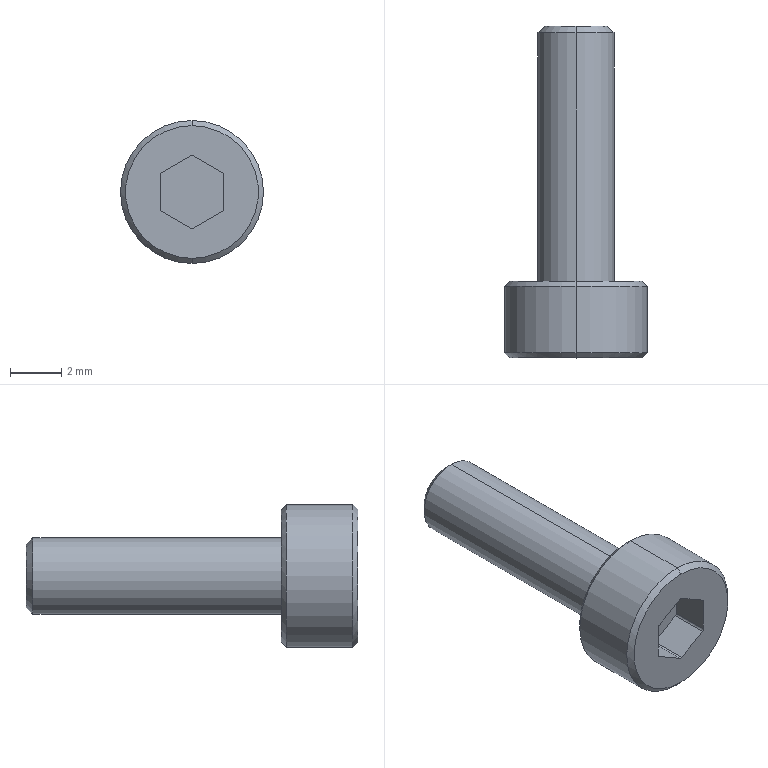Part | SolidWorks | features Chamfer 1, Extrusion 1, Fillet 1, ICE 1, StudWizard 1 | 1 solid | 27 faces | box 5.6 x 13 x 5.6 mm | volume 135.451 mm3 | cylinder 11 | plane 10 | cone 6 | commonest cylinder face diameters 0.2 x7 3 x2 5.6 x2
STEP:
#1=CARTESIAN_POINT('',(0.,0.,1.428));
#2=VERTEX_POINT('',#1);
#3=CARTESIAN_POINT('',(0.05,0.,1.415));
#4=VERTEX_POINT('',#3);
#5=CARTESIAN_POINT('',(0.,0.,1.328));
#6=DIRECTION('',(0.,1.,0.));
#7=DIRECTION('',(0.,0.,1.));
#8=AXIS2_PLACEMENT_3D('',#5,#6,#7);
#9=CIRCLE('',#8,0.1);
#10=EDGE_CURVE('',#2,#4,#9,.T.);
#11=ORIENTED_EDGE('',*,*,#10,.F.);
#12=CARTESIAN_POINT('',(0.,1.5,1.428));
#13=VERTEX_POINT('',#12);
#14=CARTESIAN_POINT('',(0.,1.5,1.428));
#15=DIRECTION('',(0.,1.,0.));
#16=VECTOR('',#15,1000.);
#17=LINE('',#14,#16);
#18=EDGE_CURVE('',#2,#13,#17,.T.);
#19=ORIENTED_EDGE('',*,*,#18,.T.);
#20=CARTESIAN_POINT('',(0.05,1.5,1.415));
#21=VERTEX_POINT('',#20);
#22=CARTESIAN_POINT('',(0.,1.5,1.328));
#23=DIRECTION('',(0.,-1.,0.));
#24=DIRECTION('',(0.,0.,-1.));
#25=AXIS2_PLACEMENT_3D('',#22,#23,#24);
#26=CIRCLE('',#25,0.1);
#27=EDGE_CURVE('',#21,#13,#26,.T.);
#28=ORIENTED_EDGE('',*,*,#27,.F.);
#29=CARTESIAN_POINT('',(0.05,1.5,1.415));
#30=DIRECTION('',(0.,1.,0.));
#31=VECTOR('',#30,1000.);
#32=LINE('',#29,#31);
#33=EDGE_CURVE('',#4,#21,#32,.T.);
#34=ORIENTED_EDGE('',*,*,#33,.F.);
#35=EDGE_LOOP('',(#11,#19,#28,#34));
#36=FACE_OUTER_BOUND('',#35,.T.);
#37=CARTESIAN_POINT('',(0.,1.5,1.328));
#38=DIRECTION('',(0.,1.,0.));
#39=DIRECTION('',(0.,0.,1.));
#40=AXIS2_PLACEMENT_3D('',#37,#38,#39);
#41=CYLINDRICAL_SURFACE('',#40,0.1);
#42=ADVANCED_FACE('',(#36),#41,.F.);
#43=CARTESIAN_POINT('',(0.,0.,-2.6));
#44=VERTEX_POINT('',#43);
#45=CARTESIAN_POINT('',(0.,0.,2.6));
#46=VERTEX_POINT('',#45);
#47=CARTESIAN_POINT('',(0.,0.,0.));
#48=DIRECTION('',(0.,-1.,0.));
#49=DIRECTION('',(0.,0.,1.));
#50=AXIS2_PLACEMENT_3D('',#47,#48,#49);
#51=CIRCLE('',#50,2.6);
#52=EDGE_CURVE('',#44,#46,#51,.T.);
#53=ORIENTED_EDGE('',*,*,#52,.F.);
#54=CARTESIAN_POINT('',(0.,0.2,-2.8));
#55=VERTEX_POINT('',#54);
#56=CARTESIAN_POINT('',(0.,0.2,-2.8));
#57=DIRECTION('',(0.,0.7071,-0.7071));
#58=VECTOR('',#57,1000.);
#59=LINE('',#56,#58);
#60=EDGE_CURVE('',#44,#55,#59,.T.);
#61=ORIENTED_EDGE('',*,*,#60,.T.);
#62=CARTESIAN_POINT('',(0.,0.2,2.8));
#63=VERTEX_POINT('',#62);
#64=CARTESIAN_POINT('',(0.,0.2,0.));
#65=DIRECTION('',(0.,1.,0.));
#66=DIRECTION('',(0.,0.,1.));
#67=AXIS2_PLACEMENT_3D('',#64,#65,#66);
#68=CIRCLE('',#67,2.8);
#69=EDGE_CURVE('',#63,#55,#68,.T.);
#70=ORIENTED_EDGE('',*,*,#69,.F.);
#71=CARTESIAN_POINT('',(0.,0.2,2.8));
#72=DIRECTION('',(0.,0.7071,0.7071));
#73=VECTOR('',#72,1000.);
#74=LINE('',#71,#73);
#75=EDGE_CURVE('',#46,#63,#74,.T.);
#76=ORIENTED_EDGE('',*,*,#75,.F.);
#77=EDGE_LOOP('',(#53,#61,#70,#76));
#78=FACE_OUTER_BOUND('',#77,.T.);
#79=CARTESIAN_POINT('',(0.,0.2,0.));
#80=DIRECTION('',(0.,1.,0.));
#81=DIRECTION('',(0.,0.,1.));
#82=AXIS2_PLACEMENT_3D('',#79,#80,#81);
#83=CONICAL_SURFACE('',#82,2.8,0.7854);
#84=ADVANCED_FACE('',(#78),#83,.T.);
#85=CARTESIAN_POINT('',(0.,3.,2.6));
#86=VERTEX_POINT('',#85);
#87=CARTESIAN_POINT('',(0.,3.,-2.6));
#88=VERTEX_POINT('',#87);
#89=CARTESIAN_POINT('',(0.,3.,0.));
#90=DIRECTION('',(0.,1.,0.));
#91=DIRECTION('',(0.,0.,1.));
#92=AXIS2_PLACEMENT_3D('',#89,#90,#91);
#93=CIRCLE('',#92,2.6);
#94=EDGE_CURVE('',#86,#88,#93,.T.);
#95=ORIENTED_EDGE('',*,*,#94,.F.);
#96=CARTESIAN_POINT('',(0.,2.8,2.8));
#97=VERTEX_POINT('',#96);
#98=CARTESIAN_POINT('',(0.,3.,2.6));
#99=DIRECTION('',(0.,-0.7071,0.7071));
#100=VECTOR('',#99,1000.);
#101=LINE('',#98,#100);
#102=EDGE_CURVE('',#86,#97,#101,.T.);
#103=ORIENTED_EDGE('',*,*,#102,.T.);
#104=CARTESIAN_POINT('',(0.,2.8,-2.8));
#105=VERTEX_POINT('',#104);
#106=CARTESIAN_POINT('',(0.,2.8,0.));
#107=DIRECTION('',(0.,-1.,0.));
#108=DIRECTION('',(0.,0.,1.));
#109=AXIS2_PLACEMENT_3D('',#106,#107,#108);
#110=CIRCLE('',#109,2.8);
#111=EDGE_CURVE('',#105,#97,#110,.T.);
#112=ORIENTED_EDGE('',*,*,#111,.F.);
#113=CARTESIAN_POINT('',(0.,3.,-2.6));
#114=DIRECTION('',(0.,-0.7071,-0.7071));
#115=VECTOR('',#114,1000.);
#116=LINE('',#113,#115);
#117=EDGE_CURVE('',#88,#105,#116,.T.);
#118=ORIENTED_EDGE('',*,*,#117,.F.);
#119=EDGE_LOOP('',(#95,#103,#112,#118));
#120=FACE_OUTER_BOUND('',#119,.T.);
#121=CARTESIAN_POINT('',(0.,3.,0.));
#122=DIRECTION('',(0.,-1.,0.));
#123=DIRECTION('',(0.,0.,-1.));
#124=AXIS2_PLACEMENT_3D('',#121,#122,#123);
#125=CONICAL_SURFACE('',#124,2.6,0.7854);
#126=ADVANCED_FACE('',(#120),#125,.T.);
#127=CARTESIAN_POINT('',(0.,12.73,-1.5));
#128=VERTEX_POINT('',#127);
#129=CARTESIAN_POINT('',(0.,12.73,1.5));
#130=VERTEX_POINT('',#129);
#131=CARTESIAN_POINT('',(0.,12.73,0.));
#132=DIRECTION('',(0.,-1.,0.));
#133=DIRECTION('',(0.,0.,-1.));
#134=AXIS2_PLACEMENT_3D('',#131,#132,#133);
#135=CIRCLE('',#134,1.5);
#136=EDGE_CURVE('',#128,#130,#135,.T.);
#137=ORIENTED_EDGE('',*,*,#136,.T.);
#138=CARTESIAN_POINT('',(0.,3.,1.5));
#139=VERTEX_POINT('',#138);
#140=CARTESIAN_POINT('',(0.,3.,1.5));
#141=DIRECTION('',(0.,-1.,0.));
#142=VECTOR('',#141,1000.);
#143=LINE('',#140,#142);
#144=EDGE_CURVE('',#130,#139,#143,.T.);
#145=ORIENTED_EDGE('',*,*,#144,.T.);
#146=CARTESIAN_POINT('',(0.,3.,-1.5));
#147=VERTEX_POINT('',#146);
#148=CARTESIAN_POINT('',(0.,3.,0.));
#149=DIRECTION('',(0.,-1.,0.));
#150=DIRECTION('',(0.,0.,-1.));
#151=AXIS2_PLACEMENT_3D('',#148,#149,#150);
#152=CIRCLE('',#151,1.5);
#153=EDGE_CURVE('',#147,#139,#152,.T.);
#154=ORIENTED_EDGE('',*,*,#153,.F.);
#155=CARTESIAN_POINT('',(0.,3.,-1.5));
#156=DIRECTION('',(0.,-1.,0.));
#157=VECTOR('',#156,1000.);
#158=LINE('',#155,#157);
#159=EDGE_CURVE('',#128,#147,#158,.T.);
#160=ORIENTED_EDGE('',*,*,#159,.F.);
#161=EDGE_LOOP('',(#137,#145,#154,#160));
#162=FACE_OUTER_BOUND('',#161,.T.);
#163=CARTESIAN_POINT('',(0.,3.,0.));
#164=DIRECTION('',(0.,-1.,0.));
#165=DIRECTION('',(0.,0.,-1.));
#166=AXIS2_PLACEMENT_3D('',#163,#164,#165);
#167=CYLINDRICAL_SURFACE('',#166,1.5);
#168=ADVANCED_FACE('',(#162),#167,.T.);
#169=CARTESIAN_POINT('',(0.,13.,-1.23));
#170=VERTEX_POINT('',#169);
#171=CARTESIAN_POINT('',(0.,13.,1.23));
#172=VERTEX_POINT('',#171);
#173=CARTESIAN_POINT('',(0.,13.,0.));
#174=DIRECTION('',(0.,-1.,0.));
#175=DIRECTION('',(0.,0.,-1.));
#176=AXIS2_PLACEMENT_3D('',#173,#174,#175);
#177=CIRCLE('',#176,1.23);
#178=EDGE_CURVE('',#170,#172,#177,.T.);
#179=ORIENTED_EDGE('',*,*,#178,.T.);
#180=CARTESIAN_POINT('',(0.,12.73,1.5));
#181=DIRECTION('',(0.,-0.7071,0.7071));
#182=VECTOR('',#181,1000.);
#183=LINE('',#180,#182);
#184=EDGE_CURVE('',#172,#130,#183,.T.);
#185=ORIENTED_EDGE('',*,*,#184,.T.);
#186=ORIENTED_EDGE('',*,*,#136,.F.);
#187=CARTESIAN_POINT('',(0.,12.73,-1.5));
#188=DIRECTION('',(0.,-0.7071,-0.7071));
#189=VECTOR('',#188,1000.);
#190=LINE('',#187,#189);
#191=EDGE_CURVE('',#170,#128,#190,.T.);
#192=ORIENTED_EDGE('',*,*,#191,.F.);
#193=EDGE_LOOP('',(#179,#185,#186,#192));
#194=FACE_OUTER_BOUND('',#193,.T.);
#195=CARTESIAN_POINT('',(0.,12.73,0.));
#196=DIRECTION('',(0.,-1.,0.));
#197=DIRECTION('',(0.,0.,-1.));
#198=AXIS2_PLACEMENT_3D('',#195,#196,#197);
#199=CONICAL_SURFACE('',#198,1.5,0.7854);
#200=ADVANCED_FACE('',(#194),#199,.T.);
#201=ORIENTED_EDGE('',*,*,#111,.T.);
#202=CARTESIAN_POINT('',(0.,3.,2.8));
#203=DIRECTION('',(0.,-1.,0.));
#204=VECTOR('',#203,1000.);
#205=LINE('',#202,#204);
#206=EDGE_CURVE('',#97,#63,#205,.T.);
#207=ORIENTED_EDGE('',*,*,#206,.T.);
#208=ORIENTED_EDGE('',*,*,#69,.T.);
#209=CARTESIAN_POINT('',(0.,3.,-2.8));
#210=DIRECTION('',(0.,-1.,0.));
#211=VECTOR('',#210,1000.);
#212=LINE('',#209,#211);
#213=EDGE_CURVE('',#105,#55,#212,.T.);
#214=ORIENTED_EDGE('',*,*,#213,.F.);
#215=EDGE_LOOP('',(#201,#207,#208,#214));
#216=FACE_OUTER_BOUND('',#215,.T.);
#217=CARTESIAN_POINT('',(0.,3.,0.));
#218=DIRECTION('',(0.,-1.,0.));
#219=DIRECTION('',(0.,0.,-1.));
#220=AXIS2_PLACEMENT_3D('',#217,#218,#219);
#221=CYLINDRICAL_SURFACE('',#220,2.8);
#222=ADVANCED_FACE('',(#216),#221,.T.);
#223=ORIENTED_EDGE('',*,*,#206,.F.);
#224=CARTESIAN_POINT('',(0.,2.8,0.));
#225=DIRECTION('',(0.,-1.,0.));
#226=DIRECTION('',(0.,0.,1.));
#227=AXIS2_PLACEMENT_3D('',#224,#225,#226);
#228=CIRCLE('',#227,2.8);
#229=EDGE_CURVE('',#97,#105,#228,.T.);
#230=ORIENTED_EDGE('',*,*,#229,.T.);
#231=ORIENTED_EDGE('',*,*,#213,.T.);
#232=CARTESIAN_POINT('',(0.,0.2,0.));
#233=DIRECTION('',(0.,1.,0.));
#234=DIRECTION('',(0.,0.,1.));
#235=AXIS2_PLACEMENT_3D('',#232,#233,#234);
#236=CIRCLE('',#235,2.8);
#237=EDGE_CURVE('',#55,#63,#236,.T.);
#238=ORIENTED_EDGE('',*,*,#237,.T.);
#239=EDGE_LOOP('',(#223,#230,#231,#238));
#240=FACE_OUTER_BOUND('',#239,.T.);
#241=CARTESIAN_POINT('',(0.,3.,0.));
#242=DIRECTION('',(0.,-1.,0.));
#243=DIRECTION('',(0.,0.,-1.));
#244=AXIS2_PLACEMENT_3D('',#241,#242,#243);
#245=CYLINDRICAL_SURFACE('',#244,2.8);
#246=ADVANCED_FACE('',(#240),#245,.T.);
#247=CARTESIAN_POINT('',(0.,3.,0.));
#248=DIRECTION('',(0.,1.,0.));
#249=DIRECTION('',(0.,0.,1.));
#250=AXIS2_PLACEMENT_3D('',#247,#248,#249);
#251=CIRCLE('',#250,2.6);
#252=EDGE_CURVE('',#88,#86,#251,.T.);
#253=ORIENTED_EDGE('',*,*,#252,.T.);
#254=ORIENTED_EDGE('',*,*,#94,.T.);
#255=EDGE_LOOP('',(#253,#254));
#256=FACE_OUTER_BOUND('',#255,.T.);
#257=ORIENTED_EDGE('',*,*,#153,.T.);
#258=CARTESIAN_POINT('',(0.,3.,0.));
#259=DIRECTION('',(0.,-1.,0.));
#260=DIRECTION('',(0.,0.,-1.));
#261=AXIS2_PLACEMENT_3D('',#258,#259,#260);
#262=CIRCLE('',#261,1.5);
#263=EDGE_CURVE('',#139,#147,#262,.T.);
#264=ORIENTED_EDGE('',*,*,#263,.T.);
#265=EDGE_LOOP('',(#257,#264));
#266=FACE_BOUND('',#265,.T.);
#267=CARTESIAN_POINT('',(0.,3.,0.));
#268=DIRECTION('',(0.,1.,0.));
#269=DIRECTION('',(0.,0.,1.));
#270=AXIS2_PLACEMENT_3D('',#267,#268,#269);
#271=PLANE('',#270);
#272=ADVANCED_FACE('',(#256,#266),#271,.T.);
#273=CARTESIAN_POINT('',(0.,0.,0.));
#274=DIRECTION('',(0.,-1.,0.));
#275=DIRECTION('',(0.,0.,1.));
#276=AXIS2_PLACEMENT_3D('',#273,#274,#275);
#277=CIRCLE('',#276,2.6);
#278=EDGE_CURVE('',#46,#44,#277,.T.);
#279=ORIENTED_EDGE('',*,*,#278,.T.);
#280=ORIENTED_EDGE('',*,*,#52,.T.);
#281=EDGE_LOOP('',(#279,#280));
#282=FACE_OUTER_BOUND('',#281,.T.);
#283=CARTESIAN_POINT('',(-0.05,0.,1.415));
#284=VERTEX_POINT('',#283);
#285=CARTESIAN_POINT('',(-1.2,0.,0.7506));
#286=VERTEX_POINT('',#285);
#287=CARTESIAN_POINT('',(0.,0.,1.443));
#288=DIRECTION('',(-0.866,0.,-0.5));
#289=VECTOR('',#288,1000.);
#290=LINE('',#287,#289);
#291=EDGE_CURVE('',#284,#286,#290,.T.);
#292=ORIENTED_EDGE('',*,*,#291,.F.);
#293=CARTESIAN_POINT('',(0.,0.,1.328));
#294=DIRECTION('',(0.,1.,0.));
#295=DIRECTION('',(0.,0.,1.));
#296=AXIS2_PLACEMENT_3D('',#293,#294,#295);
#297=CIRCLE('',#296,0.1);
#298=EDGE_CURVE('',#284,#2,#297,.T.);
#299=ORIENTED_EDGE('',*,*,#298,.T.);
#300=ORIENTED_EDGE('',*,*,#10,.T.);
#301=CARTESIAN_POINT('',(1.2,0.,0.7506));
#302=VERTEX_POINT('',#301);
#303=CARTESIAN_POINT('',(1.25,0.,0.7217));
#304=DIRECTION('',(-0.866,0.,0.5));
#305=VECTOR('',#304,1000.);
#306=LINE('',#303,#305);
#307=EDGE_CURVE('',#302,#4,#306,.T.);
#308=ORIENTED_EDGE('',*,*,#307,.F.);
#309=CARTESIAN_POINT('',(1.25,0.,0.664));
#310=VERTEX_POINT('',#309);
#311=CARTESIAN_POINT('',(1.15,0.,0.664));
#312=DIRECTION('',(0.,1.,0.));
#313=DIRECTION('',(0.,0.,1.));
#314=AXIS2_PLACEMENT_3D('',#311,#312,#313);
#315=CIRCLE('',#314,0.1);
#316=EDGE_CURVE('',#302,#310,#315,.T.);
#317=ORIENTED_EDGE('',*,*,#316,.T.);
#318=CARTESIAN_POINT('',(1.25,0.,-0.664));
#319=VERTEX_POINT('',#318);
#320=CARTESIAN_POINT('',(1.25,0.,-0.7217));
#321=DIRECTION('',(0.,0.,1.));
#322=VECTOR('',#321,1000.);
#323=LINE('',#320,#322);
#324=EDGE_CURVE('',#319,#310,#323,.T.);
#325=ORIENTED_EDGE('',*,*,#324,.F.);
#326=CARTESIAN_POINT('',(1.2,0.,-0.7506));
#327=VERTEX_POINT('',#326);
#328=CARTESIAN_POINT('',(1.15,0.,-0.664));
#329=DIRECTION('',(0.,1.,0.));
#330=DIRECTION('',(0.,0.,1.));
#331=AXIS2_PLACEMENT_3D('',#328,#329,#330);
#332=CIRCLE('',#331,0.1);
#333=EDGE_CURVE('',#319,#327,#332,.T.);
#334=ORIENTED_EDGE('',*,*,#333,.T.);
#335=CARTESIAN_POINT('',(0.05,0.,-1.415));
#336=VERTEX_POINT('',#335);
#337=CARTESIAN_POINT('',(0.,0.,-1.443));
#338=DIRECTION('',(0.866,0.,0.5));
#339=VECTOR('',#338,1000.);
#340=LINE('',#337,#339);
#341=EDGE_CURVE('',#336,#327,#340,.T.);
#342=ORIENTED_EDGE('',*,*,#341,.F.);
#343=CARTESIAN_POINT('',(-0.05,0.,-1.415));
#344=VERTEX_POINT('',#343);
#345=CARTESIAN_POINT('',(0.,0.,-1.328));
#346=DIRECTION('',(0.,1.,0.));
#347=DIRECTION('',(0.,0.,1.));
#348=AXIS2_PLACEMENT_3D('',#345,#346,#347);
#349=CIRCLE('',#348,0.1);
#350=EDGE_CURVE('',#336,#344,#349,.T.);
#351=ORIENTED_EDGE('',*,*,#350,.T.);
#352=CARTESIAN_POINT('',(-1.2,0.,-0.7506));
#353=VERTEX_POINT('',#352);
#354=CARTESIAN_POINT('',(-1.25,0.,-0.7217));
#355=DIRECTION('',(0.866,0.,-0.5));
#356=VECTOR('',#355,1000.);
#357=LINE('',#354,#356);
#358=EDGE_CURVE('',#353,#344,#357,.T.);
#359=ORIENTED_EDGE('',*,*,#358,.F.);
#360=CARTESIAN_POINT('',(-1.25,0.,-0.664));
#361=VERTEX_POINT('',#360);
#362=CARTESIAN_POINT('',(-1.15,0.,-0.664));
#363=DIRECTION('',(0.,1.,0.));
#364=DIRECTION('',(0.,0.,1.));
#365=AXIS2_PLACEMENT_3D('',#362,#363,#364);
#366=CIRCLE('',#365,0.1);
#367=EDGE_CURVE('',#353,#361,#366,.T.);
#368=ORIENTED_EDGE('',*,*,#367,.T.);
#369=CARTESIAN_POINT('',(-1.25,0.,0.664));
#370=VERTEX_POINT('',#369);
#371=CARTESIAN_POINT('',(-1.25,0.,0.7217));
#372=DIRECTION('',(0.,0.,-1.));
#373=VECTOR('',#372,1000.);
#374=LINE('',#371,#373);
#375=EDGE_CURVE('',#370,#361,#374,.T.);
#376=ORIENTED_EDGE('',*,*,#375,.F.);
#377=CARTESIAN_POINT('',(-1.15,0.,0.664));
#378=DIRECTION('',(0.,1.,0.));
#379=DIRECTION('',(0.,0.,1.));
#380=AXIS2_PLACEMENT_3D('',#377,#378,#379);
#381=CIRCLE('',#380,0.1);
#382=EDGE_CURVE('',#370,#286,#381,.T.);
#383=ORIENTED_EDGE('',*,*,#382,.T.);
#384=EDGE_LOOP('',(#292,#299,#300,#308,#317,#325,#334,#342,#351,#359,#368,#376,#383));
#385=FACE_BOUND('',#384,.T.);
#386=CARTESIAN_POINT('',(0.,0.,0.));
#387=DIRECTION('',(0.,1.,0.));
#388=DIRECTION('',(0.,0.,1.));
#389=AXIS2_PLACEMENT_3D('',#386,#387,#388);
#390=PLANE('',#389);
#391=ADVANCED_FACE('',(#282,#385),#390,.F.);
#392=ORIENTED_EDGE('',*,*,#178,.F.);
#393=CARTESIAN_POINT('',(0.,13.,0.));
#394=DIRECTION('',(0.,-1.,0.));
#395=DIRECTION('',(0.,0.,-1.));
#396=AXIS2_PLACEMENT_3D('',#393,#394,#395);
#397=CIRCLE('',#396,1.23);
#398=EDGE_CURVE('',#172,#170,#397,.T.);
#399=ORIENTED_EDGE('',*,*,#398,.F.);
#400=EDGE_LOOP('',(#392,#399));
#401=FACE_OUTER_BOUND('',#400,.T.);
#402=CARTESIAN_POINT('',(1.23,13.,0.));
#403=DIRECTION('',(0.,1.,0.));
#404=DIRECTION('',(0.,0.,1.));
#405=AXIS2_PLACEMENT_3D('',#402,#403,#404);
#406=PLANE('',#405);
#407=ADVANCED_FACE('',(#401),#406,.T.);
#408=ORIENTED_EDGE('',*,*,#184,.F.);
#409=ORIENTED_EDGE('',*,*,#398,.T.);
#410=ORIENTED_EDGE('',*,*,#191,.T.);
#411=CARTESIAN_POINT('',(0.,12.73,0.));
#412=DIRECTION('',(0.,-1.,0.));
#413=DIRECTION('',(0.,0.,-1.));
#414=AXIS2_PLACEMENT_3D('',#411,#412,#413);
#415=CIRCLE('',#414,1.5);
#416=EDGE_CURVE('',#130,#128,#415,.T.);
#417=ORIENTED_EDGE('',*,*,#416,.F.);
#418=EDGE_LOOP('',(#408,#409,#410,#417));
#419=FACE_OUTER_BOUND('',#418,.T.);
#420=CARTESIAN_POINT('',(0.,12.73,0.));
#421=DIRECTION('',(0.,-1.,0.));
#422=DIRECTION('',(0.,0.,-1.));
#423=AXIS2_PLACEMENT_3D('',#420,#421,#422);
#424=CONICAL_SURFACE('',#423,1.5,0.7854);
#425=ADVANCED_FACE('',(#419),#424,.T.);
#426=ORIENTED_EDGE('',*,*,#144,.F.);
#427=ORIENTED_EDGE('',*,*,#416,.T.);
#428=ORIENTED_EDGE('',*,*,#159,.T.);
#429=ORIENTED_EDGE('',*,*,#263,.F.);
#430=EDGE_LOOP('',(#426,#427,#428,#429));
#431=FACE_OUTER_BOUND('',#430,.T.);
#432=CARTESIAN_POINT('',(0.,3.,0.));
#433=DIRECTION('',(0.,-1.,0.));
#434=DIRECTION('',(0.,0.,-1.));
#435=AXIS2_PLACEMENT_3D('',#432,#433,#434);
#436=CYLINDRICAL_SURFACE('',#435,1.5);
#437=ADVANCED_FACE('',(#431),#436,.T.);
#438=CARTESIAN_POINT('',(1.2,1.5,0.7506));
#439=VERTEX_POINT('',#438);
#440=CARTESIAN_POINT('',(1.25,1.5,0.7217));
#441=DIRECTION('',(-0.866,0.,0.5));
#442=VECTOR('',#441,1000.);
#443=LINE('',#440,#442);
#444=EDGE_CURVE('',#439,#21,#443,.T.);
#445=ORIENTED_EDGE('',*,*,#444,.F.);
#446=CARTESIAN_POINT('',(1.2,0.,0.7506));
#447=DIRECTION('',(0.,-1.,0.));
#448=VECTOR('',#447,1000.);
#449=LINE('',#446,#448);
#450=EDGE_CURVE('',#439,#302,#449,.T.);
#451=ORIENTED_EDGE('',*,*,#450,.T.);
#452=ORIENTED_EDGE('',*,*,#307,.T.);
#453=ORIENTED_EDGE('',*,*,#33,.T.);
#454=EDGE_LOOP('',(#445,#451,#452,#453));
#455=FACE_OUTER_BOUND('',#454,.T.);
#456=CARTESIAN_POINT('',(1.25,1.5,0.7217));
#457=DIRECTION('',(0.5,0.,0.866));
#458=DIRECTION('',(0.866,0.,-0.5));
#459=AXIS2_PLACEMENT_3D('',#456,#457,#458);
#460=PLANE('',#459);
#461=ADVANCED_FACE('',(#455),#460,.F.);
#462=CARTESIAN_POINT('',(1.25,1.5,-0.664));
#463=VERTEX_POINT('',#462);
#464=CARTESIAN_POINT('',(1.25,1.5,0.664));
#465=VERTEX_POINT('',#464);
#466=CARTESIAN_POINT('',(1.25,1.5,-0.7217));
#467=DIRECTION('',(0.,0.,1.));
#468=VECTOR('',#467,1000.);
#469=LINE('',#466,#468);
#470=EDGE_CURVE('',#463,#465,#469,.T.);
#471=ORIENTED_EDGE('',*,*,#470,.F.);
#472=CARTESIAN_POINT('',(1.25,0.,-0.664));
#473=DIRECTION('',(0.,-1.,0.));
#474=VECTOR('',#473,1000.);
#475=LINE('',#472,#474);
#476=EDGE_CURVE('',#463,#319,#475,.T.);
#477=ORIENTED_EDGE('',*,*,#476,.T.);
#478=ORIENTED_EDGE('',*,*,#324,.T.);
#479=CARTESIAN_POINT('',(1.25,1.5,0.664));
#480=DIRECTION('',(0.,1.,0.));
#481=VECTOR('',#480,1000.);
#482=LINE('',#479,#481);
#483=EDGE_CURVE('',#310,#465,#482,.T.);
#484=ORIENTED_EDGE('',*,*,#483,.T.);
#485=EDGE_LOOP('',(#471,#477,#478,#484));
#486=FACE_OUTER_BOUND('',#485,.T.);
#487=CARTESIAN_POINT('',(1.25,1.5,-0.7217));
#488=DIRECTION('',(1.,0.,0.));
#489=DIRECTION('',(0.,0.,-1.));
#490=AXIS2_PLACEMENT_3D('',#487,#488,#489);
#491=PLANE('',#490);
#492=ADVANCED_FACE('',(#486),#491,.F.);
#493=CARTESIAN_POINT('',(0.05,1.5,-1.415));
#494=VERTEX_POINT('',#493);
#495=CARTESIAN_POINT('',(1.2,1.5,-0.7506));
#496=VERTEX_POINT('',#495);
#497=CARTESIAN_POINT('',(0.,1.5,-1.443));
#498=DIRECTION('',(0.866,0.,0.5));
#499=VECTOR('',#498,1000.);
#500=LINE('',#497,#499);
#501=EDGE_CURVE('',#494,#496,#500,.T.);
#502=ORIENTED_EDGE('',*,*,#501,.F.);
#503=CARTESIAN_POINT('',(0.05,0.,-1.415));
#504=DIRECTION('',(0.,-1.,0.));
#505=VECTOR('',#504,1000.);
#506=LINE('',#503,#505);
#507=EDGE_CURVE('',#494,#336,#506,.T.);
#508=ORIENTED_EDGE('',*,*,#507,.T.);
#509=ORIENTED_EDGE('',*,*,#341,.T.);
#510=CARTESIAN_POINT('',(1.2,1.5,-0.7506));
#511=DIRECTION('',(0.,1.,0.));
#512=VECTOR('',#511,1000.);
#513=LINE('',#510,#512);
#514=EDGE_CURVE('',#327,#496,#513,.T.);
#515=ORIENTED_EDGE('',*,*,#514,.T.);
#516=EDGE_LOOP('',(#502,#508,#509,#515));
#517=FACE_OUTER_BOUND('',#516,.T.);
#518=CARTESIAN_POINT('',(0.,1.5,-1.443));
#519=DIRECTION('',(0.5,0.,-0.866));
#520=DIRECTION('',(-0.866,0.,-0.5));
#521=AXIS2_PLACEMENT_3D('',#518,#519,#520);
#522=PLANE('',#521);
#523=ADVANCED_FACE('',(#517),#522,.F.);
#524=CARTESIAN_POINT('',(-1.2,1.5,-0.7506));
#525=VERTEX_POINT('',#524);
#526=CARTESIAN_POINT('',(-0.05,1.5,-1.415));
#527=VERTEX_POINT('',#526);
#528=CARTESIAN_POINT('',(-1.25,1.5,-0.7217));
#529=DIRECTION('',(0.866,0.,-0.5));
#530=VECTOR('',#529,1000.);
#531=LINE('',#528,#530);
#532=EDGE_CURVE('',#525,#527,#531,.T.);
#533=ORIENTED_EDGE('',*,*,#532,.F.);
#534=CARTESIAN_POINT('',(-1.2,0.,-0.7506));
#535=DIRECTION('',(0.,-1.,0.));
#536=VECTOR('',#535,1000.);
#537=LINE('',#534,#536);
#538=EDGE_CURVE('',#525,#353,#537,.T.);
#539=ORIENTED_EDGE('',*,*,#538,.T.);
#540=ORIENTED_EDGE('',*,*,#358,.T.);
#541=CARTESIAN_POINT('',(-0.05,1.5,-1.415));
#542=DIRECTION('',(0.,1.,0.));
#543=VECTOR('',#542,1000.);
#544=LINE('',#541,#543);
#545=EDGE_CURVE('',#344,#527,#544,.T.);
#546=ORIENTED_EDGE('',*,*,#545,.T.);
#547=EDGE_LOOP('',(#533,#539,#540,#546));
#548=FACE_OUTER_BOUND('',#547,.T.);
#549=CARTESIAN_POINT('',(-1.25,1.5,-0.7217));
#550=DIRECTION('',(-0.5,0.,-0.866));
#551=DIRECTION('',(-0.866,0.,0.5));
#552=AXIS2_PLACEMENT_3D('',#549,#550,#551);
#553=PLANE('',#552);
#554=ADVANCED_FACE('',(#548),#553,.F.);
#555=CARTESIAN_POINT('',(-1.25,1.5,0.664));
#556=VERTEX_POINT('',#555);
#557=CARTESIAN_POINT('',(-1.25,1.5,-0.664));
#558=VERTEX_POINT('',#557);
#559=CARTESIAN_POINT('',(-1.25,1.5,0.7217));
#560=DIRECTION('',(0.,0.,-1.));
#561=VECTOR('',#560,1000.);
#562=LINE('',#559,#561);
#563=EDGE_CURVE('',#556,#558,#562,.T.);
#564=ORIENTED_EDGE('',*,*,#563,.F.);
#565=CARTESIAN_POINT('',(-1.25,0.,0.664));
#566=DIRECTION('',(0.,-1.,0.));
#567=VECTOR('',#566,1000.);
#568=LINE('',#565,#567);
#569=EDGE_CURVE('',#556,#370,#568,.T.);
#570=ORIENTED_EDGE('',*,*,#569,.T.);
#571=ORIENTED_EDGE('',*,*,#375,.T.);
#572=CARTESIAN_POINT('',(-1.25,1.5,-0.664));
#573=DIRECTION('',(0.,1.,0.));
#574=VECTOR('',#573,1000.);
#575=LINE('',#572,#574);
#576=EDGE_CURVE('',#361,#558,#575,.T.);
#577=ORIENTED_EDGE('',*,*,#576,.T.);
#578=EDGE_LOOP('',(#564,#570,#571,#577));
#579=FACE_OUTER_BOUND('',#578,.T.);
#580=CARTESIAN_POINT('',(-1.25,1.5,0.7217));
#581=DIRECTION('',(-1.,0.,0.));
#582=DIRECTION('',(0.,0.,1.));
#583=AXIS2_PLACEMENT_3D('',#580,#581,#582);
#584=PLANE('',#583);
#585=ADVANCED_FACE('',(#579),#584,.F.);
#586=ORIENTED_EDGE('',*,*,#291,.T.);
#587=CARTESIAN_POINT('',(-1.2,1.5,0.7506));
#588=VERTEX_POINT('',#587);
#589=CARTESIAN_POINT('',(-1.2,1.5,0.7506));
#590=DIRECTION('',(0.,1.,0.));
#591=VECTOR('',#590,1000.);
#592=LINE('',#589,#591);
#593=EDGE_CURVE('',#286,#588,#592,.T.);
#594=ORIENTED_EDGE('',*,*,#593,.T.);
#595=CARTESIAN_POINT('',(-0.05,1.5,1.415));
#596=VERTEX_POINT('',#595);
#597=CARTESIAN_POINT('',(0.,1.5,1.443));
#598=DIRECTION('',(-0.866,0.,-0.5));
#599=VECTOR('',#598,1000.);
#600=LINE('',#597,#599);
#601=EDGE_CURVE('',#596,#588,#600,.T.);
#602=ORIENTED_EDGE('',*,*,#601,.F.);
#603=CARTESIAN_POINT('',(-0.05,0.,1.415));
#604=DIRECTION('',(0.,-1.,0.));
#605=VECTOR('',#604,1000.);
#606=LINE('',#603,#605);
#607=EDGE_CURVE('',#596,#284,#606,.T.);
#608=ORIENTED_EDGE('',*,*,#607,.T.);
#609=EDGE_LOOP('',(#586,#594,#602,#608));
#610=FACE_OUTER_BOUND('',#609,.T.);
#611=CARTESIAN_POINT('',(0.,1.5,1.443));
#612=DIRECTION('',(-0.5,0.,0.866));
#613=DIRECTION('',(0.866,0.,0.5));
#614=AXIS2_PLACEMENT_3D('',#611,#612,#613);
#615=PLANE('',#614);
#616=ADVANCED_FACE('',(#610),#615,.F.);
#617=ORIENTED_EDGE('',*,*,#601,.T.);
#618=CARTESIAN_POINT('',(-1.15,1.5,0.664));
#619=DIRECTION('',(0.,-1.,0.));
#620=DIRECTION('',(0.,0.,-1.));
#621=AXIS2_PLACEMENT_3D('',#618,#619,#620);
#622=CIRCLE('',#621,0.1);
#623=EDGE_CURVE('',#588,#556,#622,.T.);
#624=ORIENTED_EDGE('',*,*,#623,.T.);
#625=ORIENTED_EDGE('',*,*,#563,.T.);
#626=CARTESIAN_POINT('',(-1.15,1.5,-0.664));
#627=DIRECTION('',(0.,-1.,0.));
#628=DIRECTION('',(0.,0.,-1.));
#629=AXIS2_PLACEMENT_3D('',#626,#627,#628);
#630=CIRCLE('',#629,0.1);
#631=EDGE_CURVE('',#558,#525,#630,.T.);
#632=ORIENTED_EDGE('',*,*,#631,.T.);
#633=ORIENTED_EDGE('',*,*,#532,.T.);
#634=CARTESIAN_POINT('',(0.,1.5,-1.328));
#635=DIRECTION('',(0.,-1.,0.));
#636=DIRECTION('',(0.,0.,-1.));
#637=AXIS2_PLACEMENT_3D('',#634,#635,#636);
#638=CIRCLE('',#637,0.1);
#639=EDGE_CURVE('',#527,#494,#638,.T.);
#640=ORIENTED_EDGE('',*,*,#639,.T.);
#641=ORIENTED_EDGE('',*,*,#501,.T.);
#642=CARTESIAN_POINT('',(1.15,1.5,-0.664));
#643=DIRECTION('',(0.,-1.,0.));
#644=DIRECTION('',(0.,0.,-1.));
#645=AXIS2_PLACEMENT_3D('',#642,#643,#644);
#646=CIRCLE('',#645,0.1);
#647=EDGE_CURVE('',#496,#463,#646,.T.);
#648=ORIENTED_EDGE('',*,*,#647,.T.);
#649=ORIENTED_EDGE('',*,*,#470,.T.);
#650=CARTESIAN_POINT('',(1.15,1.5,0.664));
#651=DIRECTION('',(0.,-1.,0.));
#652=DIRECTION('',(0.,0.,-1.));
#653=AXIS2_PLACEMENT_3D('',#650,#651,#652);
#654=CIRCLE('',#653,0.1);
#655=EDGE_CURVE('',#465,#439,#654,.T.);
#656=ORIENTED_EDGE('',*,*,#655,.T.);
#657=ORIENTED_EDGE('',*,*,#444,.T.);
#658=ORIENTED_EDGE('',*,*,#27,.T.);
#659=CARTESIAN_POINT('',(0.,1.5,1.328));
#660=DIRECTION('',(0.,-1.,0.));
#661=DIRECTION('',(0.,0.,-1.));
#662=AXIS2_PLACEMENT_3D('',#659,#660,#661);
#663=CIRCLE('',#662,0.1);
#664=EDGE_CURVE('',#13,#596,#663,.T.);
#665=ORIENTED_EDGE('',*,*,#664,.T.);
#666=EDGE_LOOP('',(#617,#624,#625,#632,#633,#640,#641,#648,#649,#656,#657,#658,#665));
#667=FACE_OUTER_BOUND('',#666,.T.);
#668=CARTESIAN_POINT('',(0.,1.5,0.));
#669=DIRECTION('',(0.,-1.,0.));
#670=DIRECTION('',(0.,0.,-1.));
#671=AXIS2_PLACEMENT_3D('',#668,#669,#670);
#672=PLANE('',#671);
#673=ADVANCED_FACE('',(#667),#672,.T.);
#674=ORIENTED_EDGE('',*,*,#102,.F.);
#675=ORIENTED_EDGE('',*,*,#252,.F.);
#676=ORIENTED_EDGE('',*,*,#117,.T.);
#677=ORIENTED_EDGE('',*,*,#229,.F.);
#678=EDGE_LOOP('',(#674,#675,#676,#677));
#679=FACE_OUTER_BOUND('',#678,.T.);
#680=CARTESIAN_POINT('',(0.,3.,0.));
#681=DIRECTION('',(0.,-1.,0.));
#682=DIRECTION('',(0.,0.,-1.));
#683=AXIS2_PLACEMENT_3D('',#680,#681,#682);
#684=CONICAL_SURFACE('',#683,2.6,0.7854);
#685=ADVANCED_FACE('',(#679),#684,.T.);
#686=ORIENTED_EDGE('',*,*,#60,.F.);
#687=ORIENTED_EDGE('',*,*,#278,.F.);
#688=ORIENTED_EDGE('',*,*,#75,.T.);
#689=ORIENTED_EDGE('',*,*,#237,.F.);
#690=EDGE_LOOP('',(#686,#687,#688,#689));
#691=FACE_OUTER_BOUND('',#690,.T.);
#692=CARTESIAN_POINT('',(0.,0.2,0.));
#693=DIRECTION('',(0.,1.,0.));
#694=DIRECTION('',(0.,0.,1.));
#695=AXIS2_PLACEMENT_3D('',#692,#693,#694);
#696=CONICAL_SURFACE('',#695,2.8,0.7854);
#697=ADVANCED_FACE('',(#691),#696,.T.);
#698=ORIENTED_EDGE('',*,*,#623,.F.);
#699=ORIENTED_EDGE('',*,*,#593,.F.);
#700=ORIENTED_EDGE('',*,*,#382,.F.);
#701=ORIENTED_EDGE('',*,*,#569,.F.);
#702=EDGE_LOOP('',(#698,#699,#700,#701));
#703=FACE_OUTER_BOUND('',#702,.T.);
#704=CARTESIAN_POINT('',(-1.15,1.5,0.664));
#705=DIRECTION('',(0.,1.,0.));
#706=DIRECTION('',(0.,0.,1.));
#707=AXIS2_PLACEMENT_3D('',#704,#705,#706);
#708=CYLINDRICAL_SURFACE('',#707,0.1);
#709=ADVANCED_FACE('',(#703),#708,.F.);
#710=ORIENTED_EDGE('',*,*,#631,.F.);
#711=ORIENTED_EDGE('',*,*,#576,.F.);
#712=ORIENTED_EDGE('',*,*,#367,.F.);
#713=ORIENTED_EDGE('',*,*,#538,.F.);
#714=EDGE_LOOP('',(#710,#711,#712,#713));
#715=FACE_OUTER_BOUND('',#714,.T.);
#716=CARTESIAN_POINT('',(-1.15,1.5,-0.664));
#717=DIRECTION('',(0.,1.,0.));
#718=DIRECTION('',(0.,0.,1.));
#719=AXIS2_PLACEMENT_3D('',#716,#717,#718);
#720=CYLINDRICAL_SURFACE('',#719,0.1);
#721=ADVANCED_FACE('',(#715),#720,.F.);
#722=ORIENTED_EDGE('',*,*,#639,.F.);
#723=ORIENTED_EDGE('',*,*,#545,.F.);
#724=ORIENTED_EDGE('',*,*,#350,.F.);
#725=ORIENTED_EDGE('',*,*,#507,.F.);
#726=EDGE_LOOP('',(#722,#723,#724,#725));
#727=FACE_OUTER_BOUND('',#726,.T.);
#728=CARTESIAN_POINT('',(0.,1.5,-1.328));
#729=DIRECTION('',(0.,1.,0.));
#730=DIRECTION('',(0.,0.,1.));
#731=AXIS2_PLACEMENT_3D('',#728,#729,#730);
#732=CYLINDRICAL_SURFACE('',#731,0.1);
#733=ADVANCED_FACE('',(#727),#732,.F.);
#734=ORIENTED_EDGE('',*,*,#647,.F.);
#735=ORIENTED_EDGE('',*,*,#514,.F.);
#736=ORIENTED_EDGE('',*,*,#333,.F.);
#737=ORIENTED_EDGE('',*,*,#476,.F.);
#738=EDGE_LOOP('',(#734,#735,#736,#737));
#739=FACE_OUTER_BOUND('',#738,.T.);
#740=CARTESIAN_POINT('',(1.15,1.5,-0.664));
#741=DIRECTION('',(0.,1.,0.));
#742=DIRECTION('',(0.,0.,1.));
#743=AXIS2_PLACEMENT_3D('',#740,#741,#742);
#744=CYLINDRICAL_SURFACE('',#743,0.1);
#745=ADVANCED_FACE('',(#739),#744,.F.);
#746=ORIENTED_EDGE('',*,*,#655,.F.);
#747=ORIENTED_EDGE('',*,*,#483,.F.);
#748=ORIENTED_EDGE('',*,*,#316,.F.);
#749=ORIENTED_EDGE('',*,*,#450,.F.);
#750=EDGE_LOOP('',(#746,#747,#748,#749));
#751=FACE_OUTER_BOUND('',#750,.T.);
#752=CARTESIAN_POINT('',(1.15,1.5,0.664));
#753=DIRECTION('',(0.,1.,0.));
#754=DIRECTION('',(0.,0.,1.));
#755=AXIS2_PLACEMENT_3D('',#752,#753,#754);
#756=CYLINDRICAL_SURFACE('',#755,0.1);
#757=ADVANCED_FACE('',(#751),#756,.F.);
#758=ORIENTED_EDGE('',*,*,#18,.F.);
#759=ORIENTED_EDGE('',*,*,#298,.F.);
#760=ORIENTED_EDGE('',*,*,#607,.F.);
#761=ORIENTED_EDGE('',*,*,#664,.F.);
#762=EDGE_LOOP('',(#758,#759,#760,#761));
#763=FACE_OUTER_BOUND('',#762,.T.);
#764=CARTESIAN_POINT('',(0.,1.5,1.328));
#765=DIRECTION('',(0.,1.,0.));
#766=DIRECTION('',(0.,0.,1.));
#767=AXIS2_PLACEMENT_3D('',#764,#765,#766);
#768=CYLINDRICAL_SURFACE('',#767,0.1);
#769=ADVANCED_FACE('',(#763),#768,.F.);
#770=CLOSED_SHELL('',(#42,#84,#126,#168,#200,#222,#246,#272,#391,#407,#425,#437,#461,#492,#523,#554,#585,#616,#673,#685,#697,#709,#721,#733,#745,#757,#769));
#771=MANIFOLD_SOLID_BREP('',#770);
#772=CARTESIAN_POINT('',(0.,0.,0.));
#773=DIRECTION('',(0.,0.,1.));
#774=DIRECTION('',(1.,0.,0.));
#775=AXIS2_PLACEMENT_3D('',#772,#773,#774);
#776=(LENGTH_UNIT()NAMED_UNIT(*)SI_UNIT(.MILLI.,.METRE.));
#777=UNCERTAINTY_MEASURE_WITH_UNIT(LENGTH_MEASURE(0.00001),#776,'','');
#778=(NAMED_UNIT(*)PLANE_ANGLE_UNIT()SI_UNIT($,.RADIAN.));
#779=(NAMED_UNIT(*)SI_UNIT($,.STERADIAN.)SOLID_ANGLE_UNIT());
#780=(GEOMETRIC_REPRESENTATION_CONTEXT(3)GLOBAL_UNCERTAINTY_ASSIGNED_CONTEXT((#777))GLOBAL_UNIT_ASSIGNED_CONTEXT((#776,#778,#779))REPRESENTATION_CONTEXT('',''));
#781=ADVANCED_BREP_SHAPE_REPRESENTATION('',(#771,#775),#780);